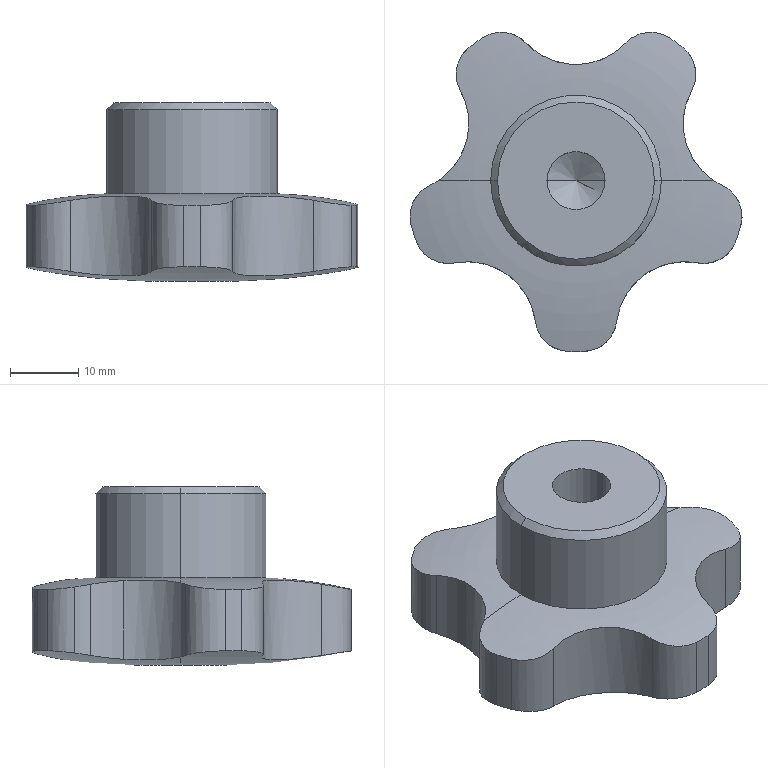Part | SolidWorks | features Chamfer 1, CirPattern 1, Fillet 1, HoleWzd 1, ICE 1, Revolution 1 | 1 solid | 36 faces | box 48.607 x 46.741 x 26.101 mm | volume 21839 mm3 | cylinder 27 | cone 4 | torus 4 | plane 1 | commonest cylinder face diameters 10 x12 20 x6 50 x5 8.5 x2 25 x2